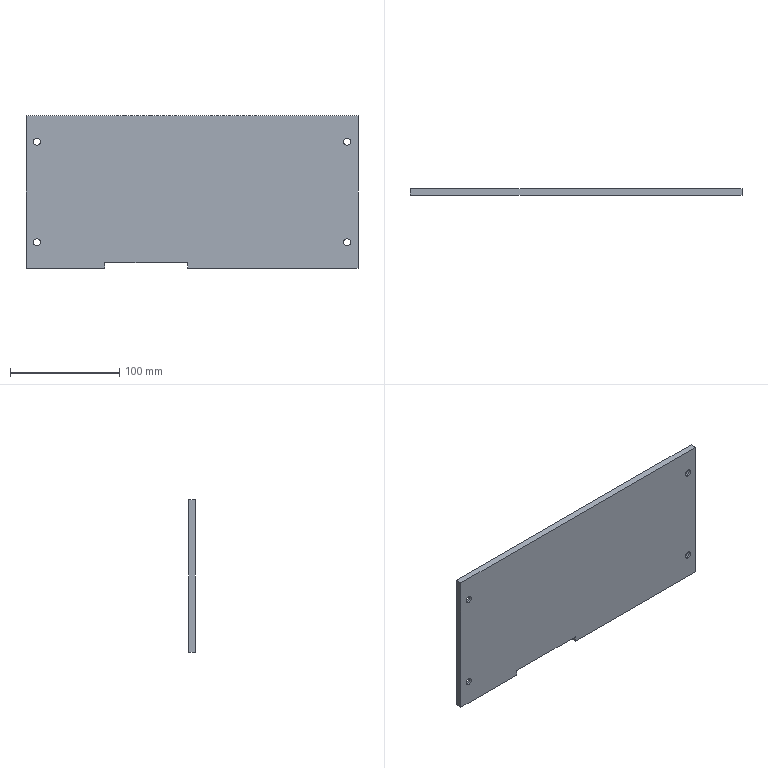Part | Creo | 1 solid | 42 faces | box 304 x 6 x 139.5 mm | volume 250207 mm3 | cone 16 | cylinder 16 | plane 10 | commonest cylinder face diameters 6.6 x8 13 x8
STEP:
#1=CARTESIAN_POINT('',(0.,0.,0.));
#2=DIRECTION('',(0.,0.,1.));
#3=DIRECTION('',(1.,0.,0.));
#4=AXIS2_PLACEMENT_3D('',#1,#2,#3);
#5=CARTESIAN_POINT('',(-4.,244.,-260.5));
#6=VERTEX_POINT('',#5);
#7=CARTESIAN_POINT('',(-4.,250.,-260.5));
#8=VERTEX_POINT('',#7);
#9=CARTESIAN_POINT('',(-4.,244.,-260.5));
#10=DIRECTION('',(0.,1.,0.));
#11=VECTOR('',#10,6.);
#12=LINE('',#9,#11);
#13=EDGE_CURVE('',#6,#8,#12,.T.);
#14=ORIENTED_EDGE('',*,*,#13,.F.);
#15=CARTESIAN_POINT('',(152.,244.,-260.5));
#16=VERTEX_POINT('',#15);
#17=CARTESIAN_POINT('',(-4.,244.,-260.5));
#18=DIRECTION('',(1.,0.,0.));
#19=VECTOR('',#18,156.);
#20=LINE('',#17,#19);
#21=EDGE_CURVE('',#6,#16,#20,.T.);
#22=ORIENTED_EDGE('',*,*,#21,.T.);
#23=CARTESIAN_POINT('',(152.,250.,-260.5));
#24=VERTEX_POINT('',#23);
#25=CARTESIAN_POINT('',(152.,244.,-260.5));
#26=DIRECTION('',(0.,1.,0.));
#27=VECTOR('',#26,6.);
#28=LINE('',#25,#27);
#29=EDGE_CURVE('',#16,#24,#28,.T.);
#30=ORIENTED_EDGE('',*,*,#29,.T.);
#31=CARTESIAN_POINT('',(152.,250.,-260.5));
#32=DIRECTION('',(-1.,0.,0.));
#33=VECTOR('',#32,156.);
#34=LINE('',#31,#33);
#35=EDGE_CURVE('',#24,#8,#34,.T.);
#36=ORIENTED_EDGE('',*,*,#35,.T.);
#37=EDGE_LOOP('',(#14,#22,#30,#36));
#38=FACE_OUTER_BOUND('',#37,.F.);
#39=CARTESIAN_POINT('',(-200.,250.,-260.5));
#40=DIRECTION('',(0.,0.,-1.));
#41=DIRECTION('',(1.,0.,0.));
#42=AXIS2_PLACEMENT_3D('',#39,#40,#41);
#43=PLANE('',#42);
#44=ADVANCED_FACE('',(#38),#43,.T.);
#45=CARTESIAN_POINT('',(-4.,244.,-255.5));
#46=VERTEX_POINT('',#45);
#47=CARTESIAN_POINT('',(-4.,244.,-255.5));
#48=DIRECTION('',(0.,0.,-1.));
#49=VECTOR('',#48,5.);
#50=LINE('',#47,#49);
#51=EDGE_CURVE('',#46,#6,#50,.T.);
#52=ORIENTED_EDGE('',*,*,#51,.T.);
#53=ORIENTED_EDGE('',*,*,#13,.T.);
#54=CARTESIAN_POINT('',(-4.,250.,-255.5));
#55=VERTEX_POINT('',#54);
#56=CARTESIAN_POINT('',(-4.,250.,-260.5));
#57=DIRECTION('',(0.,0.,1.));
#58=VECTOR('',#57,5.);
#59=LINE('',#56,#58);
#60=EDGE_CURVE('',#8,#55,#59,.T.);
#61=ORIENTED_EDGE('',*,*,#60,.T.);
#62=CARTESIAN_POINT('',(-4.,244.,-255.5));
#63=DIRECTION('',(0.,1.,0.));
#64=VECTOR('',#63,6.);
#65=LINE('',#62,#64);
#66=EDGE_CURVE('',#46,#55,#65,.T.);
#67=ORIENTED_EDGE('',*,*,#66,.F.);
#68=EDGE_LOOP('',(#52,#53,#61,#67));
#69=FACE_OUTER_BOUND('',#68,.F.);
#70=CARTESIAN_POINT('',(-4.,229.,-276.75));
#71=DIRECTION('',(1.,0.,0.));
#72=DIRECTION('',(0.,0.,-1.));
#73=AXIS2_PLACEMENT_3D('',#70,#71,#72);
#74=PLANE('',#73);
#75=ADVANCED_FACE('',(#69),#74,.F.);
#76=ORIENTED_EDGE('',*,*,#51,.F.);
#77=CARTESIAN_POINT('',(-80.,244.,-255.5));
#78=VERTEX_POINT('',#77);
#79=CARTESIAN_POINT('',(-80.,244.,-255.5));
#80=DIRECTION('',(1.,0.,0.));
#81=VECTOR('',#80,76.);
#82=LINE('',#79,#81);
#83=EDGE_CURVE('',#78,#46,#82,.T.);
#84=ORIENTED_EDGE('',*,*,#83,.F.);
#85=CARTESIAN_POINT('',(-80.,244.,-260.5));
#86=VERTEX_POINT('',#85);
#87=CARTESIAN_POINT('',(-80.,244.,-260.5));
#88=DIRECTION('',(0.,0.,1.));
#89=VECTOR('',#88,5.);
#90=LINE('',#87,#89);
#91=EDGE_CURVE('',#86,#78,#90,.T.);
#92=ORIENTED_EDGE('',*,*,#91,.F.);
#93=CARTESIAN_POINT('',(-152.,244.,-260.5));
#94=VERTEX_POINT('',#93);
#95=CARTESIAN_POINT('',(-152.,244.,-260.5));
#96=DIRECTION('',(1.,0.,0.));
#97=VECTOR('',#96,72.);
#98=LINE('',#95,#97);
#99=EDGE_CURVE('',#94,#86,#98,.T.);
#100=ORIENTED_EDGE('',*,*,#99,.F.);
#101=CARTESIAN_POINT('',(-152.,244.,-121.));
#102=VERTEX_POINT('',#101);
#103=CARTESIAN_POINT('',(-152.,244.,-121.));
#104=DIRECTION('',(0.,0.,-1.));
#105=VECTOR('',#104,139.5);
#106=LINE('',#103,#105);
#107=EDGE_CURVE('',#102,#94,#106,.T.);
#108=ORIENTED_EDGE('',*,*,#107,.F.);
#109=CARTESIAN_POINT('',(152.,244.,-121.));
#110=VERTEX_POINT('',#109);
#111=CARTESIAN_POINT('',(152.,244.,-121.));
#112=DIRECTION('',(-1.,0.,0.));
#113=VECTOR('',#112,304.);
#114=LINE('',#111,#113);
#115=EDGE_CURVE('',#110,#102,#114,.T.);
#116=ORIENTED_EDGE('',*,*,#115,.F.);
#117=CARTESIAN_POINT('',(152.,244.,-260.5));
#118=DIRECTION('',(0.,0.,1.));
#119=VECTOR('',#118,139.5);
#120=LINE('',#117,#119);
#121=EDGE_CURVE('',#16,#110,#120,.T.);
#122=ORIENTED_EDGE('',*,*,#121,.F.);
#123=ORIENTED_EDGE('',*,*,#21,.F.);
#124=EDGE_LOOP('',(#76,#84,#92,#100,#108,#116,#122,#123));
#125=FACE_OUTER_BOUND('',#124,.F.);
#126=CARTESIAN_POINT('',(-142.,244.,-240.05));
#127=VERTEX_POINT('',#126);
#128=CARTESIAN_POINT('',(-142.,244.,-233.45));
#129=VERTEX_POINT('',#128);
#130=CARTESIAN_POINT('',(-142.,244.,-236.75));
#131=DIRECTION('',(0.,1.,0.));
#132=DIRECTION('',(0.,0.,-1.));
#133=AXIS2_PLACEMENT_3D('',#130,#131,#132);
#134=CIRCLE('',#133,3.3);
#135=EDGE_CURVE('',#127,#129,#134,.T.);
#136=ORIENTED_EDGE('',*,*,#135,.F.);
#137=CARTESIAN_POINT('',(-142.,244.,-236.75));
#138=DIRECTION('',(0.,1.,0.));
#139=DIRECTION('',(0.,0.,1.));
#140=AXIS2_PLACEMENT_3D('',#137,#138,#139);
#141=CIRCLE('',#140,3.3);
#142=EDGE_CURVE('',#129,#127,#141,.T.);
#143=ORIENTED_EDGE('',*,*,#142,.F.);
#144=EDGE_LOOP('',(#136,#143));
#145=FACE_BOUND('',#144,.F.);
#146=CARTESIAN_POINT('',(-142.,244.,-148.05));
#147=VERTEX_POINT('',#146);
#148=CARTESIAN_POINT('',(-142.,244.,-141.45));
#149=VERTEX_POINT('',#148);
#150=CARTESIAN_POINT('',(-142.,244.,-144.75));
#151=DIRECTION('',(0.,1.,0.));
#152=DIRECTION('',(0.,0.,-1.));
#153=AXIS2_PLACEMENT_3D('',#150,#151,#152);
#154=CIRCLE('',#153,3.3);
#155=EDGE_CURVE('',#147,#149,#154,.T.);
#156=ORIENTED_EDGE('',*,*,#155,.F.);
#157=CARTESIAN_POINT('',(-142.,244.,-144.75));
#158=DIRECTION('',(0.,1.,0.));
#159=DIRECTION('',(0.,0.,1.));
#160=AXIS2_PLACEMENT_3D('',#157,#158,#159);
#161=CIRCLE('',#160,3.3);
#162=EDGE_CURVE('',#149,#147,#161,.T.);
#163=ORIENTED_EDGE('',*,*,#162,.F.);
#164=EDGE_LOOP('',(#156,#163));
#165=FACE_BOUND('',#164,.F.);
#166=CARTESIAN_POINT('',(142.,244.,-240.05));
#167=VERTEX_POINT('',#166);
#168=CARTESIAN_POINT('',(142.,244.,-233.45));
#169=VERTEX_POINT('',#168);
#170=CARTESIAN_POINT('',(142.,244.,-236.75));
#171=DIRECTION('',(0.,1.,0.));
#172=DIRECTION('',(0.,0.,-1.));
#173=AXIS2_PLACEMENT_3D('',#170,#171,#172);
#174=CIRCLE('',#173,3.3);
#175=EDGE_CURVE('',#167,#169,#174,.T.);
#176=ORIENTED_EDGE('',*,*,#175,.F.);
#177=CARTESIAN_POINT('',(142.,244.,-236.75));
#178=DIRECTION('',(0.,1.,0.));
#179=DIRECTION('',(0.,0.,1.));
#180=AXIS2_PLACEMENT_3D('',#177,#178,#179);
#181=CIRCLE('',#180,3.3);
#182=EDGE_CURVE('',#169,#167,#181,.T.);
#183=ORIENTED_EDGE('',*,*,#182,.F.);
#184=EDGE_LOOP('',(#176,#183));
#185=FACE_BOUND('',#184,.F.);
#186=CARTESIAN_POINT('',(142.,244.,-148.05));
#187=VERTEX_POINT('',#186);
#188=CARTESIAN_POINT('',(142.,244.,-141.45));
#189=VERTEX_POINT('',#188);
#190=CARTESIAN_POINT('',(142.,244.,-144.75));
#191=DIRECTION('',(0.,1.,0.));
#192=DIRECTION('',(0.,0.,-1.));
#193=AXIS2_PLACEMENT_3D('',#190,#191,#192);
#194=CIRCLE('',#193,3.3);
#195=EDGE_CURVE('',#187,#189,#194,.T.);
#196=ORIENTED_EDGE('',*,*,#195,.F.);
#197=CARTESIAN_POINT('',(142.,244.,-144.75));
#198=DIRECTION('',(0.,1.,0.));
#199=DIRECTION('',(0.,0.,1.));
#200=AXIS2_PLACEMENT_3D('',#197,#198,#199);
#201=CIRCLE('',#200,3.3);
#202=EDGE_CURVE('',#189,#187,#201,.T.);
#203=ORIENTED_EDGE('',*,*,#202,.F.);
#204=EDGE_LOOP('',(#196,#203));
#205=FACE_BOUND('',#204,.F.);
#206=CARTESIAN_POINT('',(0.,244.,-193.5));
#207=DIRECTION('',(0.,-1.,0.));
#208=DIRECTION('',(0.,0.,-1.));
#209=AXIS2_PLACEMENT_3D('',#206,#207,#208);
#210=PLANE('',#209);
#211=ADVANCED_FACE('',(#125,#145,#165,#185,#205),#210,.T.);
#212=ORIENTED_EDGE('',*,*,#83,.T.);
#213=ORIENTED_EDGE('',*,*,#66,.T.);
#214=CARTESIAN_POINT('',(-80.,250.,-255.5));
#215=VERTEX_POINT('',#214);
#216=CARTESIAN_POINT('',(-4.,250.,-255.5));
#217=DIRECTION('',(-1.,0.,0.));
#218=VECTOR('',#217,76.);
#219=LINE('',#216,#218);
#220=EDGE_CURVE('',#55,#215,#219,.T.);
#221=ORIENTED_EDGE('',*,*,#220,.T.);
#222=CARTESIAN_POINT('',(-80.,244.,-255.5));
#223=DIRECTION('',(0.,1.,0.));
#224=VECTOR('',#223,6.);
#225=LINE('',#222,#224);
#226=EDGE_CURVE('',#78,#215,#225,.T.);
#227=ORIENTED_EDGE('',*,*,#226,.F.);
#228=EDGE_LOOP('',(#212,#213,#221,#227));
#229=FACE_OUTER_BOUND('',#228,.F.);
#230=CARTESIAN_POINT('',(-40.75,236.,-255.5));
#231=DIRECTION('',(0.,0.,1.));
#232=DIRECTION('',(1.,0.,0.));
#233=AXIS2_PLACEMENT_3D('',#230,#231,#232);
#234=PLANE('',#233);
#235=ADVANCED_FACE('',(#229),#234,.F.);
#236=ORIENTED_EDGE('',*,*,#60,.F.);
#237=ORIENTED_EDGE('',*,*,#35,.F.);
#238=CARTESIAN_POINT('',(152.,250.,-121.));
#239=VERTEX_POINT('',#238);
#240=CARTESIAN_POINT('',(152.,250.,-121.));
#241=DIRECTION('',(0.,0.,-1.));
#242=VECTOR('',#241,139.5);
#243=LINE('',#240,#242);
#244=EDGE_CURVE('',#239,#24,#243,.T.);
#245=ORIENTED_EDGE('',*,*,#244,.F.);
#246=CARTESIAN_POINT('',(-152.,250.,-121.));
#247=VERTEX_POINT('',#246);
#248=CARTESIAN_POINT('',(-152.,250.,-121.));
#249=DIRECTION('',(1.,0.,0.));
#250=VECTOR('',#249,304.);
#251=LINE('',#248,#250);
#252=EDGE_CURVE('',#247,#239,#251,.T.);
#253=ORIENTED_EDGE('',*,*,#252,.F.);
#254=CARTESIAN_POINT('',(-152.,250.,-260.5));
#255=VERTEX_POINT('',#254);
#256=CARTESIAN_POINT('',(-152.,250.,-260.5));
#257=DIRECTION('',(0.,0.,1.));
#258=VECTOR('',#257,139.5);
#259=LINE('',#256,#258);
#260=EDGE_CURVE('',#255,#247,#259,.T.);
#261=ORIENTED_EDGE('',*,*,#260,.F.);
#262=CARTESIAN_POINT('',(-80.,250.,-260.5));
#263=VERTEX_POINT('',#262);
#264=CARTESIAN_POINT('',(-80.,250.,-260.5));
#265=DIRECTION('',(-1.,0.,0.));
#266=VECTOR('',#265,72.);
#267=LINE('',#264,#266);
#268=EDGE_CURVE('',#263,#255,#267,.T.);
#269=ORIENTED_EDGE('',*,*,#268,.F.);
#270=CARTESIAN_POINT('',(-80.,250.,-255.5));
#271=DIRECTION('',(0.,0.,-1.));
#272=VECTOR('',#271,5.);
#273=LINE('',#270,#272);
#274=EDGE_CURVE('',#215,#263,#273,.T.);
#275=ORIENTED_EDGE('',*,*,#274,.F.);
#276=ORIENTED_EDGE('',*,*,#220,.F.);
#277=EDGE_LOOP('',(#236,#237,#245,#253,#261,#269,#275,#276));
#278=FACE_OUTER_BOUND('',#277,.F.);
#279=CARTESIAN_POINT('',(-142.,250.,-243.5));
#280=VERTEX_POINT('',#279);
#281=CARTESIAN_POINT('',(-142.,250.,-230.));
#282=VERTEX_POINT('',#281);
#283=CARTESIAN_POINT('',(-142.,250.,-236.75));
#284=DIRECTION('',(0.,-1.,0.));
#285=DIRECTION('',(0.,0.,-1.));
#286=AXIS2_PLACEMENT_3D('',#283,#284,#285);
#287=CIRCLE('',#286,6.75);
#288=EDGE_CURVE('',#280,#282,#287,.T.);
#289=ORIENTED_EDGE('',*,*,#288,.F.);
#290=CARTESIAN_POINT('',(-142.,250.,-236.75));
#291=DIRECTION('',(0.,-1.,0.));
#292=DIRECTION('',(0.,0.,1.));
#293=AXIS2_PLACEMENT_3D('',#290,#291,#292);
#294=CIRCLE('',#293,6.75);
#295=EDGE_CURVE('',#282,#280,#294,.T.);
#296=ORIENTED_EDGE('',*,*,#295,.F.);
#297=EDGE_LOOP('',(#289,#296));
#298=FACE_BOUND('',#297,.F.);
#299=CARTESIAN_POINT('',(-142.,250.,-151.5));
#300=VERTEX_POINT('',#299);
#301=CARTESIAN_POINT('',(-142.,250.,-138.));
#302=VERTEX_POINT('',#301);
#303=CARTESIAN_POINT('',(-142.,250.,-144.75));
#304=DIRECTION('',(0.,-1.,0.));
#305=DIRECTION('',(0.,0.,-1.));
#306=AXIS2_PLACEMENT_3D('',#303,#304,#305);
#307=CIRCLE('',#306,6.75);
#308=EDGE_CURVE('',#300,#302,#307,.T.);
#309=ORIENTED_EDGE('',*,*,#308,.F.);
#310=CARTESIAN_POINT('',(-142.,250.,-144.75));
#311=DIRECTION('',(0.,-1.,0.));
#312=DIRECTION('',(0.,0.,1.));
#313=AXIS2_PLACEMENT_3D('',#310,#311,#312);
#314=CIRCLE('',#313,6.75);
#315=EDGE_CURVE('',#302,#300,#314,.T.);
#316=ORIENTED_EDGE('',*,*,#315,.F.);
#317=EDGE_LOOP('',(#309,#316));
#318=FACE_BOUND('',#317,.F.);
#319=CARTESIAN_POINT('',(142.,250.,-243.5));
#320=VERTEX_POINT('',#319);
#321=CARTESIAN_POINT('',(142.,250.,-230.));
#322=VERTEX_POINT('',#321);
#323=CARTESIAN_POINT('',(142.,250.,-236.75));
#324=DIRECTION('',(0.,-1.,0.));
#325=DIRECTION('',(0.,0.,-1.));
#326=AXIS2_PLACEMENT_3D('',#323,#324,#325);
#327=CIRCLE('',#326,6.75);
#328=EDGE_CURVE('',#320,#322,#327,.T.);
#329=ORIENTED_EDGE('',*,*,#328,.F.);
#330=CARTESIAN_POINT('',(142.,250.,-236.75));
#331=DIRECTION('',(0.,-1.,0.));
#332=DIRECTION('',(0.,0.,1.));
#333=AXIS2_PLACEMENT_3D('',#330,#331,#332);
#334=CIRCLE('',#333,6.75);
#335=EDGE_CURVE('',#322,#320,#334,.T.);
#336=ORIENTED_EDGE('',*,*,#335,.F.);
#337=EDGE_LOOP('',(#329,#336));
#338=FACE_BOUND('',#337,.F.);
#339=CARTESIAN_POINT('',(142.,250.,-151.5));
#340=VERTEX_POINT('',#339);
#341=CARTESIAN_POINT('',(142.,250.,-138.));
#342=VERTEX_POINT('',#341);
#343=CARTESIAN_POINT('',(142.,250.,-144.75));
#344=DIRECTION('',(0.,-1.,0.));
#345=DIRECTION('',(0.,0.,-1.));
#346=AXIS2_PLACEMENT_3D('',#343,#344,#345);
#347=CIRCLE('',#346,6.75);
#348=EDGE_CURVE('',#340,#342,#347,.T.);
#349=ORIENTED_EDGE('',*,*,#348,.F.);
#350=CARTESIAN_POINT('',(142.,250.,-144.75));
#351=DIRECTION('',(0.,-1.,0.));
#352=DIRECTION('',(0.,0.,1.));
#353=AXIS2_PLACEMENT_3D('',#350,#351,#352);
#354=CIRCLE('',#353,6.75);
#355=EDGE_CURVE('',#342,#340,#354,.T.);
#356=ORIENTED_EDGE('',*,*,#355,.F.);
#357=EDGE_LOOP('',(#349,#356));
#358=FACE_BOUND('',#357,.F.);
#359=CARTESIAN_POINT('',(-200.,250.,-260.5));
#360=DIRECTION('',(0.,-1.,0.));
#361=DIRECTION('',(0.,0.,1.));
#362=AXIS2_PLACEMENT_3D('',#359,#360,#361);
#363=PLANE('',#362);
#364=ADVANCED_FACE('',(#278,#298,#318,#338,#358),#363,.F.);
#365=ORIENTED_EDGE('',*,*,#244,.T.);
#366=ORIENTED_EDGE('',*,*,#29,.F.);
#367=ORIENTED_EDGE('',*,*,#121,.T.);
#368=CARTESIAN_POINT('',(152.,244.,-121.));
#369=DIRECTION('',(0.,1.,0.));
#370=VECTOR('',#369,6.);
#371=LINE('',#368,#370);
#372=EDGE_CURVE('',#110,#239,#371,.T.);
#373=ORIENTED_EDGE('',*,*,#372,.T.);
#374=EDGE_LOOP('',(#365,#366,#367,#373));
#375=FACE_OUTER_BOUND('',#374,.F.);
#376=CARTESIAN_POINT('',(152.,-250.,-260.5));
#377=DIRECTION('',(1.,0.,0.));
#378=DIRECTION('',(0.,0.,1.));
#379=AXIS2_PLACEMENT_3D('',#376,#377,#378);
#380=PLANE('',#379);
#381=ADVANCED_FACE('',(#375),#380,.T.);
#382=CARTESIAN_POINT('',(-152.,244.,-121.));
#383=DIRECTION('',(0.,1.,0.));
#384=VECTOR('',#383,6.);
#385=LINE('',#382,#384);
#386=EDGE_CURVE('',#102,#247,#385,.T.);
#387=ORIENTED_EDGE('',*,*,#386,.T.);
#388=ORIENTED_EDGE('',*,*,#252,.T.);
#389=ORIENTED_EDGE('',*,*,#372,.F.);
#390=ORIENTED_EDGE('',*,*,#115,.T.);
#391=EDGE_LOOP('',(#387,#388,#389,#390));
#392=FACE_OUTER_BOUND('',#391,.F.);
#393=CARTESIAN_POINT('',(-200.,250.,-121.));
#394=DIRECTION('',(0.,0.,-1.));
#395=DIRECTION('',(1.,0.,0.));
#396=AXIS2_PLACEMENT_3D('',#393,#394,#395);
#397=PLANE('',#396);
#398=ADVANCED_FACE('',(#392),#397,.F.);
#399=CARTESIAN_POINT('',(-152.,244.,-260.5));
#400=DIRECTION('',(0.,1.,0.));
#401=VECTOR('',#400,6.);
#402=LINE('',#399,#401);
#403=EDGE_CURVE('',#94,#255,#402,.T.);
#404=ORIENTED_EDGE('',*,*,#403,.T.);
#405=ORIENTED_EDGE('',*,*,#260,.T.);
#406=ORIENTED_EDGE('',*,*,#386,.F.);
#407=ORIENTED_EDGE('',*,*,#107,.T.);
#408=EDGE_LOOP('',(#404,#405,#406,#407));
#409=FACE_OUTER_BOUND('',#408,.F.);
#410=CARTESIAN_POINT('',(-152.,250.,-260.5));
#411=DIRECTION('',(-1.,0.,0.));
#412=DIRECTION('',(0.,1.,0.));
#413=AXIS2_PLACEMENT_3D('',#410,#411,#412);
#414=PLANE('',#413);
#415=ADVANCED_FACE('',(#409),#414,.T.);
#416=CARTESIAN_POINT('',(-80.,250.,-260.5));
#417=DIRECTION('',(0.,-1.,0.));
#418=VECTOR('',#417,6.);
#419=LINE('',#416,#418);
#420=EDGE_CURVE('',#263,#86,#419,.T.);
#421=ORIENTED_EDGE('',*,*,#420,.F.);
#422=ORIENTED_EDGE('',*,*,#268,.T.);
#423=ORIENTED_EDGE('',*,*,#403,.F.);
#424=ORIENTED_EDGE('',*,*,#99,.T.);
#425=EDGE_LOOP('',(#421,#422,#423,#424));
#426=FACE_OUTER_BOUND('',#425,.F.);
#427=CARTESIAN_POINT('',(-200.,250.,-260.5));
#428=DIRECTION('',(0.,0.,-1.));
#429=DIRECTION('',(1.,0.,0.));
#430=AXIS2_PLACEMENT_3D('',#427,#428,#429);
#431=PLANE('',#430);
#432=ADVANCED_FACE('',(#426),#431,.T.);
#433=ORIENTED_EDGE('',*,*,#91,.T.);
#434=ORIENTED_EDGE('',*,*,#226,.T.);
#435=ORIENTED_EDGE('',*,*,#274,.T.);
#436=ORIENTED_EDGE('',*,*,#420,.T.);
#437=EDGE_LOOP('',(#433,#434,#435,#436));
#438=FACE_OUTER_BOUND('',#437,.F.);
#439=CARTESIAN_POINT('',(-80.,229.,-276.75));
#440=DIRECTION('',(-1.,0.,0.));
#441=DIRECTION('',(0.,0.,1.));
#442=AXIS2_PLACEMENT_3D('',#439,#440,#441);
#443=PLANE('',#442);
#444=ADVANCED_FACE('',(#438),#443,.F.);
#445=ORIENTED_EDGE('',*,*,#288,.T.);
#446=CARTESIAN_POINT('',(-142.,249.75,-230.25));
#447=VERTEX_POINT('',#446);
#448=CARTESIAN_POINT('',(-142.,249.75,-230.25));
#449=DIRECTION('',(0.,0.7071,0.7071));
#450=VECTOR('',#449,0.3536);
#451=LINE('',#448,#450);
#452=EDGE_CURVE('',#447,#282,#451,.T.);
#453=ORIENTED_EDGE('',*,*,#452,.F.);
#454=CARTESIAN_POINT('',(-135.5,249.75,-236.75));
#455=VERTEX_POINT('',#454);
#456=CARTESIAN_POINT('',(-142.,249.75,-236.75));
#457=DIRECTION('',(0.,-1.,0.));
#458=DIRECTION('',(1.,0.,0.));
#459=AXIS2_PLACEMENT_3D('',#456,#457,#458);
#460=CIRCLE('',#459,6.5);
#461=EDGE_CURVE('',#455,#447,#460,.T.);
#462=ORIENTED_EDGE('',*,*,#461,.F.);
#463=CARTESIAN_POINT('',(-142.,249.75,-243.25));
#464=VERTEX_POINT('',#463);
#465=CARTESIAN_POINT('',(-142.,249.75,-236.75));
#466=DIRECTION('',(0.,-1.,0.));
#467=DIRECTION('',(0.,0.,-1.));
#468=AXIS2_PLACEMENT_3D('',#465,#466,#467);
#469=CIRCLE('',#468,6.5);
#470=EDGE_CURVE('',#464,#455,#469,.T.);
#471=ORIENTED_EDGE('',*,*,#470,.F.);
#472=CARTESIAN_POINT('',(-142.,249.75,-243.25));
#473=DIRECTION('',(0.,0.7071,-0.7071));
#474=VECTOR('',#473,0.3536);
#475=LINE('',#472,#474);
#476=EDGE_CURVE('',#464,#280,#475,.T.);
#477=ORIENTED_EDGE('',*,*,#476,.T.);
#478=EDGE_LOOP('',(#445,#453,#462,#471,#477));
#479=FACE_OUTER_BOUND('',#478,.F.);
#480=CARTESIAN_POINT('',(-142.,249.875,-236.75));
#481=DIRECTION('',(0.,1.,0.));
#482=DIRECTION('',(0.,0.,1.));
#483=AXIS2_PLACEMENT_3D('',#480,#481,#482);
#484=CONICAL_SURFACE('',#483,6.625,45.);
#485=ADVANCED_FACE('',(#479),#484,.F.);
#486=ORIENTED_EDGE('',*,*,#295,.T.);
#487=ORIENTED_EDGE('',*,*,#476,.F.);
#488=CARTESIAN_POINT('',(-148.5,249.75,-236.75));
#489=VERTEX_POINT('',#488);
#490=CARTESIAN_POINT('',(-142.,249.75,-236.75));
#491=DIRECTION('',(0.,-1.,0.));
#492=DIRECTION('',(-1.,0.,0.));
#493=AXIS2_PLACEMENT_3D('',#490,#491,#492);
#494=CIRCLE('',#493,6.5);
#495=EDGE_CURVE('',#489,#464,#494,.T.);
#496=ORIENTED_EDGE('',*,*,#495,.F.);
#497=CARTESIAN_POINT('',(-142.,249.75,-236.75));
#498=DIRECTION('',(0.,-1.,0.));
#499=DIRECTION('',(0.,0.,1.));
#500=AXIS2_PLACEMENT_3D('',#497,#498,#499);
#501=CIRCLE('',#500,6.5);
#502=EDGE_CURVE('',#447,#489,#501,.T.);
#503=ORIENTED_EDGE('',*,*,#502,.F.);
#504=ORIENTED_EDGE('',*,*,#452,.T.);
#505=EDGE_LOOP('',(#486,#487,#496,#503,#504));
#506=FACE_OUTER_BOUND('',#505,.F.);
#507=CARTESIAN_POINT('',(-142.,249.875,-236.75));
#508=DIRECTION('',(0.,1.,0.));
#509=DIRECTION('',(0.,0.,1.));
#510=AXIS2_PLACEMENT_3D('',#507,#508,#509);
#511=CONICAL_SURFACE('',#510,6.625,45.);
#512=ADVANCED_FACE('',(#506),#511,.F.);
#513=CARTESIAN_POINT('',(-135.5,248.26,-236.75));
#514=VERTEX_POINT('',#513);
#515=CARTESIAN_POINT('',(-148.5,248.26,-236.75));
#516=VERTEX_POINT('',#515);
#517=CARTESIAN_POINT('',(-142.,248.26,-236.75));
#518=DIRECTION('',(0.,1.,0.));
#519=DIRECTION('',(1.,0.,0.));
#520=AXIS2_PLACEMENT_3D('',#517,#518,#519);
#521=CIRCLE('',#520,6.5);
#522=EDGE_CURVE('',#514,#516,#521,.T.);
#523=ORIENTED_EDGE('',*,*,#522,.T.);
#524=CARTESIAN_POINT('',(-148.5,248.26,-236.75));
#525=DIRECTION('',(0.,1.,0.));
#526=VECTOR('',#525,1.49);
#527=LINE('',#524,#526);
#528=EDGE_CURVE('',#516,#489,#527,.T.);
#529=ORIENTED_EDGE('',*,*,#528,.T.);
#530=ORIENTED_EDGE('',*,*,#495,.T.);
#531=ORIENTED_EDGE('',*,*,#470,.T.);
#532=CARTESIAN_POINT('',(-135.5,248.26,-236.75));
#533=DIRECTION('',(0.,1.,0.));
#534=VECTOR('',#533,1.49);
#535=LINE('',#532,#534);
#536=EDGE_CURVE('',#514,#455,#535,.T.);
#537=ORIENTED_EDGE('',*,*,#536,.F.);
#538=EDGE_LOOP('',(#523,#529,#530,#531,#537));
#539=FACE_OUTER_BOUND('',#538,.F.);
#540=CARTESIAN_POINT('',(-142.,250.,-236.75));
#541=DIRECTION('',(0.,1.,0.));
#542=DIRECTION('',(1.,0.,0.));
#543=AXIS2_PLACEMENT_3D('',#540,#541,#542);
#544=CYLINDRICAL_SURFACE('',#543,6.5);
#545=ADVANCED_FACE('',(#539),#544,.F.);
#546=ORIENTED_EDGE('',*,*,#522,.F.);
#547=CARTESIAN_POINT('',(-138.7,245.7,-236.75));
#548=VERTEX_POINT('',#547);
#549=CARTESIAN_POINT('',(-138.7,245.7,-236.75));
#550=DIRECTION('',(0.7809,0.6247,0.));
#551=VECTOR('',#550,4.098);
#552=LINE('',#549,#551);
#553=EDGE_CURVE('',#548,#514,#552,.T.);
#554=ORIENTED_EDGE('',*,*,#553,.F.);
#555=CARTESIAN_POINT('',(-142.,245.7,-240.05));
#556=VERTEX_POINT('',#555);
#557=CARTESIAN_POINT('',(-142.,245.7,-236.75));
#558=DIRECTION('',(0.,-1.,0.));
#559=DIRECTION('',(0.,0.,-1.));
#560=AXIS2_PLACEMENT_3D('',#557,#558,#559);
#561=CIRCLE('',#560,3.3);
#562=EDGE_CURVE('',#556,#548,#561,.T.);
#563=ORIENTED_EDGE('',*,*,#562,.F.);
#564=CARTESIAN_POINT('',(-145.3,245.7,-236.75));
#565=VERTEX_POINT('',#564);
#566=CARTESIAN_POINT('',(-142.,245.7,-236.75));
#567=DIRECTION('',(0.,-1.,0.));
#568=DIRECTION('',(-1.,0.,0.));
#569=AXIS2_PLACEMENT_3D('',#566,#567,#568);
#570=CIRCLE('',#569,3.3);
#571=EDGE_CURVE('',#565,#556,#570,.T.);
#572=ORIENTED_EDGE('',*,*,#571,.F.);
#573=CARTESIAN_POINT('',(-145.3,245.7,-236.75));
#574=DIRECTION('',(-0.7809,0.6247,0.));
#575=VECTOR('',#574,4.098);
#576=LINE('',#573,#575);
#577=EDGE_CURVE('',#565,#516,#576,.T.);
#578=ORIENTED_EDGE('',*,*,#577,.T.);
#579=EDGE_LOOP('',(#546,#554,#563,#572,#578));
#580=FACE_OUTER_BOUND('',#579,.F.);
#581=CARTESIAN_POINT('',(-142.,246.98,-236.75));
#582=DIRECTION('',(0.,1.,0.));
#583=DIRECTION('',(1.,0.,0.));
#584=AXIS2_PLACEMENT_3D('',#581,#582,#583);
#585=CONICAL_SURFACE('',#584,4.9,51.34);
#586=ADVANCED_FACE('',(#580),#585,.F.);
#587=CARTESIAN_POINT('',(-142.,248.26,-236.75));
#588=DIRECTION('',(0.,1.,0.));
#589=DIRECTION('',(-1.,0.,0.));
#590=AXIS2_PLACEMENT_3D('',#587,#588,#589);
#591=CIRCLE('',#590,6.5);
#592=EDGE_CURVE('',#516,#514,#591,.T.);
#593=ORIENTED_EDGE('',*,*,#592,.F.);
#594=ORIENTED_EDGE('',*,*,#577,.F.);
#595=CARTESIAN_POINT('',(-142.,245.7,-233.45));
#596=VERTEX_POINT('',#595);
#597=CARTESIAN_POINT('',(-142.,245.7,-236.75));
#598=DIRECTION('',(0.,-1.,0.));
#599=DIRECTION('',(0.,0.,1.));
#600=AXIS2_PLACEMENT_3D('',#597,#598,#599);
#601=CIRCLE('',#600,3.3);
#602=EDGE_CURVE('',#596,#565,#601,.T.);
#603=ORIENTED_EDGE('',*,*,#602,.F.);
#604=CARTESIAN_POINT('',(-142.,245.7,-236.75));
#605=DIRECTION('',(0.,-1.,0.));
#606=DIRECTION('',(1.,0.,0.));
#607=AXIS2_PLACEMENT_3D('',#604,#605,#606);
#608=CIRCLE('',#607,3.3);
#609=EDGE_CURVE('',#548,#596,#608,.T.);
#610=ORIENTED_EDGE('',*,*,#609,.F.);
#611=ORIENTED_EDGE('',*,*,#553,.T.);
#612=EDGE_LOOP('',(#593,#594,#603,#610,#611));
#613=FACE_OUTER_BOUND('',#612,.F.);
#614=CARTESIAN_POINT('',(-142.,246.98,-236.75));
#615=DIRECTION('',(0.,1.,0.));
#616=DIRECTION('',(1.,0.,0.));
#617=AXIS2_PLACEMENT_3D('',#614,#615,#616);
#618=CONICAL_SURFACE('',#617,4.9,51.34);
#619=ADVANCED_FACE('',(#613),#618,.F.);
#620=ORIENTED_EDGE('',*,*,#592,.T.);
#621=ORIENTED_EDGE('',*,*,#536,.T.);
#622=ORIENTED_EDGE('',*,*,#461,.T.);
#623=ORIENTED_EDGE('',*,*,#502,.T.);
#624=ORIENTED_EDGE('',*,*,#528,.F.);
#625=EDGE_LOOP('',(#620,#621,#622,#623,#624));
#626=FACE_OUTER_BOUND('',#625,.F.);
#627=CARTESIAN_POINT('',(-142.,250.,-236.75));
#628=DIRECTION('',(0.,1.,0.));
#629=DIRECTION('',(1.,0.,0.));
#630=AXIS2_PLACEMENT_3D('',#627,#628,#629);
#631=CYLINDRICAL_SURFACE('',#630,6.5);
#632=ADVANCED_FACE('',(#626),#631,.F.);
#633=ORIENTED_EDGE('',*,*,#135,.T.);
#634=CARTESIAN_POINT('',(-142.,245.7,-233.45));
#635=DIRECTION('',(0.,-1.,0.));
#636=VECTOR('',#635,1.7);
#637=LINE('',#634,#636);
#638=EDGE_CURVE('',#596,#129,#637,.T.);
#639=ORIENTED_EDGE('',*,*,#638,.F.);
#640=ORIENTED_EDGE('',*,*,#602,.T.);
#641=ORIENTED_EDGE('',*,*,#571,.T.);
#642=CARTESIAN_POINT('',(-142.,245.7,-240.05));
#643=DIRECTION('',(0.,-1.,0.));
#644=VECTOR('',#643,1.7);
#645=LINE('',#642,#644);
#646=EDGE_CURVE('',#556,#127,#645,.T.);
#647=ORIENTED_EDGE('',*,*,#646,.T.);
#648=EDGE_LOOP('',(#633,#639,#640,#641,#647));
#649=FACE_OUTER_BOUND('',#648,.F.);
#650=CARTESIAN_POINT('',(-142.,200.,-236.75));
#651=DIRECTION('',(0.,-1.,0.));
#652=DIRECTION('',(0.,0.,-1.));
#653=AXIS2_PLACEMENT_3D('',#650,#651,#652);
#654=CYLINDRICAL_SURFACE('',#653,3.3);
#655=ADVANCED_FACE('',(#649),#654,.F.);
#656=ORIENTED_EDGE('',*,*,#142,.T.);
#657=ORIENTED_EDGE('',*,*,#646,.F.);
#658=ORIENTED_EDGE('',*,*,#562,.T.);
#659=ORIENTED_EDGE('',*,*,#609,.T.);
#660=ORIENTED_EDGE('',*,*,#638,.T.);
#661=EDGE_LOOP('',(#656,#657,#658,#659,#660));
#662=FACE_OUTER_BOUND('',#661,.F.);
#663=CARTESIAN_POINT('',(-142.,200.,-236.75));
#664=DIRECTION('',(0.,-1.,0.));
#665=DIRECTION('',(0.,0.,-1.));
#666=AXIS2_PLACEMENT_3D('',#663,#664,#665);
#667=CYLINDRICAL_SURFACE('',#666,3.3);
#668=ADVANCED_FACE('',(#662),#667,.F.);
#669=ORIENTED_EDGE('',*,*,#308,.T.);
#670=CARTESIAN_POINT('',(-142.,249.75,-138.25));
#671=VERTEX_POINT('',#670);
#672=CARTESIAN_POINT('',(-142.,249.75,-138.25));
#673=DIRECTION('',(0.,0.7071,0.7071));
#674=VECTOR('',#673,0.3536);
#675=LINE('',#672,#674);
#676=EDGE_CURVE('',#671,#302,#675,.T.);
#677=ORIENTED_EDGE('',*,*,#676,.F.);
#678=CARTESIAN_POINT('',(-135.5,249.75,-144.75));
#679=VERTEX_POINT('',#678);
#680=CARTESIAN_POINT('',(-142.,249.75,-144.75));
#681=DIRECTION('',(0.,-1.,0.));
#682=DIRECTION('',(1.,0.,0.));
#683=AXIS2_PLACEMENT_3D('',#680,#681,#682);
#684=CIRCLE('',#683,6.5);
#685=EDGE_CURVE('',#679,#671,#684,.T.);
#686=ORIENTED_EDGE('',*,*,#685,.F.);
#687=CARTESIAN_POINT('',(-142.,249.75,-151.25));
#688=VERTEX_POINT('',#687);
#689=CARTESIAN_POINT('',(-142.,249.75,-144.75));
#690=DIRECTION('',(0.,-1.,0.));
#691=DIRECTION('',(0.,0.,-1.));
#692=AXIS2_PLACEMENT_3D('',#689,#690,#691);
#693=CIRCLE('',#692,6.5);
#694=EDGE_CURVE('',#688,#679,#693,.T.);
#695=ORIENTED_EDGE('',*,*,#694,.F.);
#696=CARTESIAN_POINT('',(-142.,249.75,-151.25));
#697=DIRECTION('',(0.,0.7071,-0.7071));
#698=VECTOR('',#697,0.3536);
#699=LINE('',#696,#698);
#700=EDGE_CURVE('',#688,#300,#699,.T.);
#701=ORIENTED_EDGE('',*,*,#700,.T.);
#702=EDGE_LOOP('',(#669,#677,#686,#695,#701));
#703=FACE_OUTER_BOUND('',#702,.F.);
#704=CARTESIAN_POINT('',(-142.,249.875,-144.75));
#705=DIRECTION('',(0.,1.,0.));
#706=DIRECTION('',(0.,0.,1.));
#707=AXIS2_PLACEMENT_3D('',#704,#705,#706);
#708=CONICAL_SURFACE('',#707,6.625,45.);
#709=ADVANCED_FACE('',(#703),#708,.F.);
#710=ORIENTED_EDGE('',*,*,#315,.T.);
#711=ORIENTED_EDGE('',*,*,#700,.F.);
#712=CARTESIAN_POINT('',(-148.5,249.75,-144.75));
#713=VERTEX_POINT('',#712);
#714=CARTESIAN_POINT('',(-142.,249.75,-144.75));
#715=DIRECTION('',(0.,-1.,0.));
#716=DIRECTION('',(-1.,0.,0.));
#717=AXIS2_PLACEMENT_3D('',#714,#715,#716);
#718=CIRCLE('',#717,6.5);
#719=EDGE_CURVE('',#713,#688,#718,.T.);
#720=ORIENTED_EDGE('',*,*,#719,.F.);
#721=CARTESIAN_POINT('',(-142.,249.75,-144.75));
#722=DIRECTION('',(0.,-1.,0.));
#723=DIRECTION('',(0.,0.,1.));
#724=AXIS2_PLACEMENT_3D('',#721,#722,#723);
#725=CIRCLE('',#724,6.5);
#726=EDGE_CURVE('',#671,#713,#725,.T.);
#727=ORIENTED_EDGE('',*,*,#726,.F.);
#728=ORIENTED_EDGE('',*,*,#676,.T.);
#729=EDGE_LOOP('',(#710,#711,#720,#727,#728));
#730=FACE_OUTER_BOUND('',#729,.F.);
#731=CARTESIAN_POINT('',(-142.,249.875,-144.75));
#732=DIRECTION('',(0.,1.,0.));
#733=DIRECTION('',(0.,0.,1.));
#734=AXIS2_PLACEMENT_3D('',#731,#732,#733);
#735=CONICAL_SURFACE('',#734,6.625,45.);
#736=ADVANCED_FACE('',(#730),#735,.F.);
#737=CARTESIAN_POINT('',(-135.5,248.26,-144.75));
#738=VERTEX_POINT('',#737);
#739=CARTESIAN_POINT('',(-148.5,248.26,-144.75));
#740=VERTEX_POINT('',#739);
#741=CARTESIAN_POINT('',(-142.,248.26,-144.75));
#742=DIRECTION('',(0.,1.,0.));
#743=DIRECTION('',(1.,0.,0.));
#744=AXIS2_PLACEMENT_3D('',#741,#742,#743);
#745=CIRCLE('',#744,6.5);
#746=EDGE_CURVE('',#738,#740,#745,.T.);
#747=ORIENTED_EDGE('',*,*,#746,.T.);
#748=CARTESIAN_POINT('',(-148.5,248.26,-144.75));
#749=DIRECTION('',(0.,1.,0.));
#750=VECTOR('',#749,1.49);
#751=LINE('',#748,#750);
#752=EDGE_CURVE('',#740,#713,#751,.T.);
#753=ORIENTED_EDGE('',*,*,#752,.T.);
#754=ORIENTED_EDGE('',*,*,#719,.T.);
#755=ORIENTED_EDGE('',*,*,#694,.T.);
#756=CARTESIAN_POINT('',(-135.5,248.26,-144.75));
#757=DIRECTION('',(0.,1.,0.));
#758=VECTOR('',#757,1.49);
#759=LINE('',#756,#758);
#760=EDGE_CURVE('',#738,#679,#759,.T.);
#761=ORIENTED_EDGE('',*,*,#760,.F.);
#762=EDGE_LOOP('',(#747,#753,#754,#755,#761));
#763=FACE_OUTER_BOUND('',#762,.F.);
#764=CARTESIAN_POINT('',(-142.,250.,-144.75));
#765=DIRECTION('',(0.,1.,0.));
#766=DIRECTION('',(1.,0.,0.));
#767=AXIS2_PLACEMENT_3D('',#764,#765,#766);
#768=CYLINDRICAL_SURFACE('',#767,6.5);
#769=ADVANCED_FACE('',(#763),#768,.F.);
#770=ORIENTED_EDGE('',*,*,#746,.F.);
#771=CARTESIAN_POINT('',(-138.7,245.7,-144.75));
#772=VERTEX_POINT('',#771);
#773=CARTESIAN_POINT('',(-138.7,245.7,-144.75));
#774=DIRECTION('',(0.7809,0.6247,0.));
#775=VECTOR('',#774,4.098);
#776=LINE('',#773,#775);
#777=EDGE_CURVE('',#772,#738,#776,.T.);
#778=ORIENTED_EDGE('',*,*,#777,.F.);
#779=CARTESIAN_POINT('',(-142.,245.7,-148.05));
#780=VERTEX_POINT('',#779);
#781=CARTESIAN_POINT('',(-142.,245.7,-144.75));
#782=DIRECTION('',(0.,-1.,0.));
#783=DIRECTION('',(0.,0.,-1.));
#784=AXIS2_PLACEMENT_3D('',#781,#782,#783);
#785=CIRCLE('',#784,3.3);
#786=EDGE_CURVE('',#780,#772,#785,.T.);
#787=ORIENTED_EDGE('',*,*,#786,.F.);
#788=CARTESIAN_POINT('',(-145.3,245.7,-144.75));
#789=VERTEX_POINT('',#788);
#790=CARTESIAN_POINT('',(-142.,245.7,-144.75));
#791=DIRECTION('',(0.,-1.,0.));
#792=DIRECTION('',(-1.,0.,0.));
#793=AXIS2_PLACEMENT_3D('',#790,#791,#792);
#794=CIRCLE('',#793,3.3);
#795=EDGE_CURVE('',#789,#780,#794,.T.);
#796=ORIENTED_EDGE('',*,*,#795,.F.);
#797=CARTESIAN_POINT('',(-145.3,245.7,-144.75));
#798=DIRECTION('',(-0.7809,0.6247,0.));
#799=VECTOR('',#798,4.098);
#800=LINE('',#797,#799);
#801=EDGE_CURVE('',#789,#740,#800,.T.);
#802=ORIENTED_EDGE('',*,*,#801,.T.);
#803=EDGE_LOOP('',(#770,#778,#787,#796,#802));
#804=FACE_OUTER_BOUND('',#803,.F.);
#805=CARTESIAN_POINT('',(-142.,246.98,-144.75));
#806=DIRECTION('',(0.,1.,0.));
#807=DIRECTION('',(1.,0.,0.));
#808=AXIS2_PLACEMENT_3D('',#805,#806,#807);
#809=CONICAL_SURFACE('',#808,4.9,51.34);
#810=ADVANCED_FACE('',(#804),#809,.F.);
#811=CARTESIAN_POINT('',(-142.,248.26,-144.75));
#812=DIRECTION('',(0.,1.,0.));
#813=DIRECTION('',(-1.,0.,0.));
#814=AXIS2_PLACEMENT_3D('',#811,#812,#813);
#815=CIRCLE('',#814,6.5);
#816=EDGE_CURVE('',#740,#738,#815,.T.);
#817=ORIENTED_EDGE('',*,*,#816,.F.);
#818=ORIENTED_EDGE('',*,*,#801,.F.);
#819=CARTESIAN_POINT('',(-142.,245.7,-141.45));
#820=VERTEX_POINT('',#819);
#821=CARTESIAN_POINT('',(-142.,245.7,-144.75));
#822=DIRECTION('',(0.,-1.,0.));
#823=DIRECTION('',(0.,0.,1.));
#824=AXIS2_PLACEMENT_3D('',#821,#822,#823);
#825=CIRCLE('',#824,3.3);
#826=EDGE_CURVE('',#820,#789,#825,.T.);
#827=ORIENTED_EDGE('',*,*,#826,.F.);
#828=CARTESIAN_POINT('',(-142.,245.7,-144.75));
#829=DIRECTION('',(0.,-1.,0.));
#830=DIRECTION('',(1.,0.,0.));
#831=AXIS2_PLACEMENT_3D('',#828,#829,#830);
#832=CIRCLE('',#831,3.3);
#833=EDGE_CURVE('',#772,#820,#832,.T.);
#834=ORIENTED_EDGE('',*,*,#833,.F.);
#835=ORIENTED_EDGE('',*,*,#777,.T.);
#836=EDGE_LOOP('',(#817,#818,#827,#834,#835));
#837=FACE_OUTER_BOUND('',#836,.F.);
#838=CARTESIAN_POINT('',(-142.,246.98,-144.75));
#839=DIRECTION('',(0.,1.,0.));
#840=DIRECTION('',(1.,0.,0.));
#841=AXIS2_PLACEMENT_3D('',#838,#839,#840);
#842=CONICAL_SURFACE('',#841,4.9,51.34);
#843=ADVANCED_FACE('',(#837),#842,.F.);
#844=ORIENTED_EDGE('',*,*,#816,.T.);
#845=ORIENTED_EDGE('',*,*,#760,.T.);
#846=ORIENTED_EDGE('',*,*,#685,.T.);
#847=ORIENTED_EDGE('',*,*,#726,.T.);
#848=ORIENTED_EDGE('',*,*,#752,.F.);
#849=EDGE_LOOP('',(#844,#845,#846,#847,#848));
#850=FACE_OUTER_BOUND('',#849,.F.);
#851=CARTESIAN_POINT('',(-142.,250.,-144.75));
#852=DIRECTION('',(0.,1.,0.));
#853=DIRECTION('',(1.,0.,0.));
#854=AXIS2_PLACEMENT_3D('',#851,#852,#853);
#855=CYLINDRICAL_SURFACE('',#854,6.5);
#856=ADVANCED_FACE('',(#850),#855,.F.);
#857=ORIENTED_EDGE('',*,*,#155,.T.);
#858=CARTESIAN_POINT('',(-142.,245.7,-141.45));
#859=DIRECTION('',(0.,-1.,0.));
#860=VECTOR('',#859,1.7);
#861=LINE('',#858,#860);
#862=EDGE_CURVE('',#820,#149,#861,.T.);
#863=ORIENTED_EDGE('',*,*,#862,.F.);
#864=ORIENTED_EDGE('',*,*,#826,.T.);
#865=ORIENTED_EDGE('',*,*,#795,.T.);
#866=CARTESIAN_POINT('',(-142.,245.7,-148.05));
#867=DIRECTION('',(0.,-1.,0.));
#868=VECTOR('',#867,1.7);
#869=LINE('',#866,#868);
#870=EDGE_CURVE('',#780,#147,#869,.T.);
#871=ORIENTED_EDGE('',*,*,#870,.T.);
#872=EDGE_LOOP('',(#857,#863,#864,#865,#871));
#873=FACE_OUTER_BOUND('',#872,.F.);
#874=CARTESIAN_POINT('',(-142.,200.,-144.75));
#875=DIRECTION('',(0.,-1.,0.));
#876=DIRECTION('',(0.,0.,-1.));
#877=AXIS2_PLACEMENT_3D('',#874,#875,#876);
#878=CYLINDRICAL_SURFACE('',#877,3.3);
#879=ADVANCED_FACE('',(#873),#878,.F.);
#880=ORIENTED_EDGE('',*,*,#162,.T.);
#881=ORIENTED_EDGE('',*,*,#870,.F.);
#882=ORIENTED_EDGE('',*,*,#786,.T.);
#883=ORIENTED_EDGE('',*,*,#833,.T.);
#884=ORIENTED_EDGE('',*,*,#862,.T.);
#885=EDGE_LOOP('',(#880,#881,#882,#883,#884));
#886=FACE_OUTER_BOUND('',#885,.F.);
#887=CARTESIAN_POINT('',(-142.,200.,-144.75));
#888=DIRECTION('',(0.,-1.,0.));
#889=DIRECTION('',(0.,0.,-1.));
#890=AXIS2_PLACEMENT_3D('',#887,#888,#889);
#891=CYLINDRICAL_SURFACE('',#890,3.3);
#892=ADVANCED_FACE('',(#886),#891,.F.);
#893=ORIENTED_EDGE('',*,*,#328,.T.);
#894=CARTESIAN_POINT('',(142.,249.75,-230.25));
#895=VERTEX_POINT('',#894);
#896=CARTESIAN_POINT('',(142.,249.75,-230.25));
#897=DIRECTION('',(0.,0.7071,0.7071));
#898=VECTOR('',#897,0.3536);
#899=LINE('',#896,#898);
#900=EDGE_CURVE('',#895,#322,#899,.T.);
#901=ORIENTED_EDGE('',*,*,#900,.F.);
#902=CARTESIAN_POINT('',(148.5,249.75,-236.75));
#903=VERTEX_POINT('',#902);
#904=CARTESIAN_POINT('',(142.,249.75,-236.75));
#905=DIRECTION('',(0.,-1.,0.));
#906=DIRECTION('',(1.,0.,0.));
#907=AXIS2_PLACEMENT_3D('',#904,#905,#906);
#908=CIRCLE('',#907,6.5);
#909=EDGE_CURVE('',#903,#895,#908,.T.);
#910=ORIENTED_EDGE('',*,*,#909,.F.);
#911=CARTESIAN_POINT('',(142.,249.75,-243.25));
#912=VERTEX_POINT('',#911);
#913=CARTESIAN_POINT('',(142.,249.75,-236.75));
#914=DIRECTION('',(0.,-1.,0.));
#915=DIRECTION('',(0.,0.,-1.));
#916=AXIS2_PLACEMENT_3D('',#913,#914,#915);
#917=CIRCLE('',#916,6.5);
#918=EDGE_CURVE('',#912,#903,#917,.T.);
#919=ORIENTED_EDGE('',*,*,#918,.F.);
#920=CARTESIAN_POINT('',(142.,249.75,-243.25));
#921=DIRECTION('',(0.,0.7071,-0.7071));
#922=VECTOR('',#921,0.3536);
#923=LINE('',#920,#922);
#924=EDGE_CURVE('',#912,#320,#923,.T.);
#925=ORIENTED_EDGE('',*,*,#924,.T.);
#926=EDGE_LOOP('',(#893,#901,#910,#919,#925));
#927=FACE_OUTER_BOUND('',#926,.F.);
#928=CARTESIAN_POINT('',(142.,249.875,-236.75));
#929=DIRECTION('',(0.,1.,0.));
#930=DIRECTION('',(0.,0.,1.));
#931=AXIS2_PLACEMENT_3D('',#928,#929,#930);
#932=CONICAL_SURFACE('',#931,6.625,45.);
#933=ADVANCED_FACE('',(#927),#932,.F.);
#934=ORIENTED_EDGE('',*,*,#335,.T.);
#935=ORIENTED_EDGE('',*,*,#924,.F.);
#936=CARTESIAN_POINT('',(135.5,249.75,-236.75));
#937=VERTEX_POINT('',#936);
#938=CARTESIAN_POINT('',(142.,249.75,-236.75));
#939=DIRECTION('',(0.,-1.,0.));
#940=DIRECTION('',(-1.,0.,0.));
#941=AXIS2_PLACEMENT_3D('',#938,#939,#940);
#942=CIRCLE('',#941,6.5);
#943=EDGE_CURVE('',#937,#912,#942,.T.);
#944=ORIENTED_EDGE('',*,*,#943,.F.);
#945=CARTESIAN_POINT('',(142.,249.75,-236.75));
#946=DIRECTION('',(0.,-1.,0.));
#947=DIRECTION('',(0.,0.,1.));
#948=AXIS2_PLACEMENT_3D('',#945,#946,#947);
#949=CIRCLE('',#948,6.5);
#950=EDGE_CURVE('',#895,#937,#949,.T.);
#951=ORIENTED_EDGE('',*,*,#950,.F.);
#952=ORIENTED_EDGE('',*,*,#900,.T.);
#953=EDGE_LOOP('',(#934,#935,#944,#951,#952));
#954=FACE_OUTER_BOUND('',#953,.F.);
#955=CARTESIAN_POINT('',(142.,249.875,-236.75));
#956=DIRECTION('',(0.,1.,0.));
#957=DIRECTION('',(0.,0.,1.));
#958=AXIS2_PLACEMENT_3D('',#955,#956,#957);
#959=CONICAL_SURFACE('',#958,6.625,45.);
#960=ADVANCED_FACE('',(#954),#959,.F.);
#961=CARTESIAN_POINT('',(148.5,248.26,-236.75));
#962=VERTEX_POINT('',#961);
#963=CARTESIAN_POINT('',(135.5,248.26,-236.75));
#964=VERTEX_POINT('',#963);
#965=CARTESIAN_POINT('',(142.,248.26,-236.75));
#966=DIRECTION('',(0.,1.,0.));
#967=DIRECTION('',(1.,0.,0.));
#968=AXIS2_PLACEMENT_3D('',#965,#966,#967);
#969=CIRCLE('',#968,6.5);
#970=EDGE_CURVE('',#962,#964,#969,.T.);
#971=ORIENTED_EDGE('',*,*,#970,.T.);
#972=CARTESIAN_POINT('',(135.5,248.26,-236.75));
#973=DIRECTION('',(0.,1.,0.));
#974=VECTOR('',#973,1.49);
#975=LINE('',#972,#974);
#976=EDGE_CURVE('',#964,#937,#975,.T.);
#977=ORIENTED_EDGE('',*,*,#976,.T.);
#978=ORIENTED_EDGE('',*,*,#943,.T.);
#979=ORIENTED_EDGE('',*,*,#918,.T.);
#980=CARTESIAN_POINT('',(148.5,248.26,-236.75));
#981=DIRECTION('',(0.,1.,0.));
#982=VECTOR('',#981,1.49);
#983=LINE('',#980,#982);
#984=EDGE_CURVE('',#962,#903,#983,.T.);
#985=ORIENTED_EDGE('',*,*,#984,.F.);
#986=EDGE_LOOP('',(#971,#977,#978,#979,#985));
#987=FACE_OUTER_BOUND('',#986,.F.);
#988=CARTESIAN_POINT('',(142.,250.,-236.75));
#989=DIRECTION('',(0.,1.,0.));
#990=DIRECTION('',(1.,0.,0.));
#991=AXIS2_PLACEMENT_3D('',#988,#989,#990);
#992=CYLINDRICAL_SURFACE('',#991,6.5);
#993=ADVANCED_FACE('',(#987),#992,.F.);
#994=ORIENTED_EDGE('',*,*,#970,.F.);
#995=CARTESIAN_POINT('',(145.3,245.7,-236.75));
#996=VERTEX_POINT('',#995);
#997=CARTESIAN_POINT('',(145.3,245.7,-236.75));
#998=DIRECTION('',(0.7809,0.6247,0.));
#999=VECTOR('',#998,4.098);
#1000=LINE('',#997,#999);
#1001=EDGE_CURVE('',#996,#962,#1000,.T.);
#1002=ORIENTED_EDGE('',*,*,#1001,.F.);
#1003=CARTESIAN_POINT('',(142.,245.7,-240.05));
#1004=VERTEX_POINT('',#1003);
#1005=CARTESIAN_POINT('',(142.,245.7,-236.75));
#1006=DIRECTION('',(0.,-1.,0.));
#1007=DIRECTION('',(0.,0.,-1.));
#1008=AXIS2_PLACEMENT_3D('',#1005,#1006,#1007);
#1009=CIRCLE('',#1008,3.3);
#1010=EDGE_CURVE('',#1004,#996,#1009,.T.);
#1011=ORIENTED_EDGE('',*,*,#1010,.F.);
#1012=CARTESIAN_POINT('',(138.7,245.7,-236.75));
#1013=VERTEX_POINT('',#1012);
#1014=CARTESIAN_POINT('',(142.,245.7,-236.75));
#1015=DIRECTION('',(0.,-1.,0.));
#1016=DIRECTION('',(-1.,0.,0.));
#1017=AXIS2_PLACEMENT_3D('',#1014,#1015,#1016);
#1018=CIRCLE('',#1017,3.3);
#1019=EDGE_CURVE('',#1013,#1004,#1018,.T.);
#1020=ORIENTED_EDGE('',*,*,#1019,.F.);
#1021=CARTESIAN_POINT('',(138.7,245.7,-236.75));
#1022=DIRECTION('',(-0.7809,0.6247,0.));
#1023=VECTOR('',#1022,4.098);
#1024=LINE('',#1021,#1023);
#1025=EDGE_CURVE('',#1013,#964,#1024,.T.);
#1026=ORIENTED_EDGE('',*,*,#1025,.T.);
#1027=EDGE_LOOP('',(#994,#1002,#1011,#1020,#1026));
#1028=FACE_OUTER_BOUND('',#1027,.F.);
#1029=CARTESIAN_POINT('',(142.,246.98,-236.75));
#1030=DIRECTION('',(0.,1.,0.));
#1031=DIRECTION('',(1.,0.,0.));
#1032=AXIS2_PLACEMENT_3D('',#1029,#1030,#1031);
#1033=CONICAL_SURFACE('',#1032,4.9,51.34);
#1034=ADVANCED_FACE('',(#1028),#1033,.F.);
#1035=CARTESIAN_POINT('',(142.,248.26,-236.75));
#1036=DIRECTION('',(0.,1.,0.));
#1037=DIRECTION('',(-1.,0.,0.));
#1038=AXIS2_PLACEMENT_3D('',#1035,#1036,#1037);
#1039=CIRCLE('',#1038,6.5);
#1040=EDGE_CURVE('',#964,#962,#1039,.T.);
#1041=ORIENTED_EDGE('',*,*,#1040,.F.);
#1042=ORIENTED_EDGE('',*,*,#1025,.F.);
#1043=CARTESIAN_POINT('',(142.,245.7,-233.45));
#1044=VERTEX_POINT('',#1043);
#1045=CARTESIAN_POINT('',(142.,245.7,-236.75));
#1046=DIRECTION('',(0.,-1.,0.));
#1047=DIRECTION('',(0.,0.,1.));
#1048=AXIS2_PLACEMENT_3D('',#1045,#1046,#1047);
#1049=CIRCLE('',#1048,3.3);
#1050=EDGE_CURVE('',#1044,#1013,#1049,.T.);
#1051=ORIENTED_EDGE('',*,*,#1050,.F.);
#1052=CARTESIAN_POINT('',(142.,245.7,-236.75));
#1053=DIRECTION('',(0.,-1.,0.));
#1054=DIRECTION('',(1.,0.,0.));
#1055=AXIS2_PLACEMENT_3D('',#1052,#1053,#1054);
#1056=CIRCLE('',#1055,3.3);
#1057=EDGE_CURVE('',#996,#1044,#1056,.T.);
#1058=ORIENTED_EDGE('',*,*,#1057,.F.);
#1059=ORIENTED_EDGE('',*,*,#1001,.T.);
#1060=EDGE_LOOP('',(#1041,#1042,#1051,#1058,#1059));
#1061=FACE_OUTER_BOUND('',#1060,.F.);
#1062=CARTESIAN_POINT('',(142.,246.98,-236.75));
#1063=DIRECTION('',(0.,1.,0.));
#1064=DIRECTION('',(1.,0.,0.));
#1065=AXIS2_PLACEMENT_3D('',#1062,#1063,#1064);
#1066=CONICAL_SURFACE('',#1065,4.9,51.34);
#1067=ADVANCED_FACE('',(#1061),#1066,.F.);
#1068=ORIENTED_EDGE('',*,*,#1040,.T.);
#1069=ORIENTED_EDGE('',*,*,#984,.T.);
#1070=ORIENTED_EDGE('',*,*,#909,.T.);
#1071=ORIENTED_EDGE('',*,*,#950,.T.);
#1072=ORIENTED_EDGE('',*,*,#976,.F.);
#1073=EDGE_LOOP('',(#1068,#1069,#1070,#1071,#1072));
#1074=FACE_OUTER_BOUND('',#1073,.F.);
#1075=CARTESIAN_POINT('',(142.,250.,-236.75));
#1076=DIRECTION('',(0.,1.,0.));
#1077=DIRECTION('',(1.,0.,0.));
#1078=AXIS2_PLACEMENT_3D('',#1075,#1076,#1077);
#1079=CYLINDRICAL_SURFACE('',#1078,6.5);
#1080=ADVANCED_FACE('',(#1074),#1079,.F.);
#1081=ORIENTED_EDGE('',*,*,#175,.T.);
#1082=CARTESIAN_POINT('',(142.,245.7,-233.45));
#1083=DIRECTION('',(0.,-1.,0.));
#1084=VECTOR('',#1083,1.7);
#1085=LINE('',#1082,#1084);
#1086=EDGE_CURVE('',#1044,#169,#1085,.T.);
#1087=ORIENTED_EDGE('',*,*,#1086,.F.);
#1088=ORIENTED_EDGE('',*,*,#1050,.T.);
#1089=ORIENTED_EDGE('',*,*,#1019,.T.);
#1090=CARTESIAN_POINT('',(142.,245.7,-240.05));
#1091=DIRECTION('',(0.,-1.,0.));
#1092=VECTOR('',#1091,1.7);
#1093=LINE('',#1090,#1092);
#1094=EDGE_CURVE('',#1004,#167,#1093,.T.);
#1095=ORIENTED_EDGE('',*,*,#1094,.T.);
#1096=EDGE_LOOP('',(#1081,#1087,#1088,#1089,#1095));
#1097=FACE_OUTER_BOUND('',#1096,.F.);
#1098=CARTESIAN_POINT('',(142.,200.,-236.75));
#1099=DIRECTION('',(0.,-1.,0.));
#1100=DIRECTION('',(0.,0.,-1.));
#1101=AXIS2_PLACEMENT_3D('',#1098,#1099,#1100);
#1102=CYLINDRICAL_SURFACE('',#1101,3.3);
#1103=ADVANCED_FACE('',(#1097),#1102,.F.);
#1104=ORIENTED_EDGE('',*,*,#182,.T.);
#1105=ORIENTED_EDGE('',*,*,#1094,.F.);
#1106=ORIENTED_EDGE('',*,*,#1010,.T.);
#1107=ORIENTED_EDGE('',*,*,#1057,.T.);
#1108=ORIENTED_EDGE('',*,*,#1086,.T.);
#1109=EDGE_LOOP('',(#1104,#1105,#1106,#1107,#1108));
#1110=FACE_OUTER_BOUND('',#1109,.F.);
#1111=CARTESIAN_POINT('',(142.,200.,-236.75));
#1112=DIRECTION('',(0.,-1.,0.));
#1113=DIRECTION('',(0.,0.,-1.));
#1114=AXIS2_PLACEMENT_3D('',#1111,#1112,#1113);
#1115=CYLINDRICAL_SURFACE('',#1114,3.3);
#1116=ADVANCED_FACE('',(#1110),#1115,.F.);
#1117=ORIENTED_EDGE('',*,*,#348,.T.);
#1118=CARTESIAN_POINT('',(142.,249.75,-138.25));
#1119=VERTEX_POINT('',#1118);
#1120=CARTESIAN_POINT('',(142.,249.75,-138.25));
#1121=DIRECTION('',(0.,0.7071,0.7071));
#1122=VECTOR('',#1121,0.3536);
#1123=LINE('',#1120,#1122);
#1124=EDGE_CURVE('',#1119,#342,#1123,.T.);
#1125=ORIENTED_EDGE('',*,*,#1124,.F.);
#1126=CARTESIAN_POINT('',(148.5,249.75,-144.75));
#1127=VERTEX_POINT('',#1126);
#1128=CARTESIAN_POINT('',(142.,249.75,-144.75));
#1129=DIRECTION('',(0.,-1.,0.));
#1130=DIRECTION('',(1.,0.,0.));
#1131=AXIS2_PLACEMENT_3D('',#1128,#1129,#1130);
#1132=CIRCLE('',#1131,6.5);
#1133=EDGE_CURVE('',#1127,#1119,#1132,.T.);
#1134=ORIENTED_EDGE('',*,*,#1133,.F.);
#1135=CARTESIAN_POINT('',(142.,249.75,-151.25));
#1136=VERTEX_POINT('',#1135);
#1137=CARTESIAN_POINT('',(142.,249.75,-144.75));
#1138=DIRECTION('',(0.,-1.,0.));
#1139=DIRECTION('',(0.,0.,-1.));
#1140=AXIS2_PLACEMENT_3D('',#1137,#1138,#1139);
#1141=CIRCLE('',#1140,6.5);
#1142=EDGE_CURVE('',#1136,#1127,#1141,.T.);
#1143=ORIENTED_EDGE('',*,*,#1142,.F.);
#1144=CARTESIAN_POINT('',(142.,249.75,-151.25));
#1145=DIRECTION('',(0.,0.7071,-0.7071));
#1146=VECTOR('',#1145,0.3536);
#1147=LINE('',#1144,#1146);
#1148=EDGE_CURVE('',#1136,#340,#1147,.T.);
#1149=ORIENTED_EDGE('',*,*,#1148,.T.);
#1150=EDGE_LOOP('',(#1117,#1125,#1134,#1143,#1149));
#1151=FACE_OUTER_BOUND('',#1150,.F.);
#1152=CARTESIAN_POINT('',(142.,249.875,-144.75));
#1153=DIRECTION('',(0.,1.,0.));
#1154=DIRECTION('',(0.,0.,1.));
#1155=AXIS2_PLACEMENT_3D('',#1152,#1153,#1154);
#1156=CONICAL_SURFACE('',#1155,6.625,45.);
#1157=ADVANCED_FACE('',(#1151),#1156,.F.);
#1158=ORIENTED_EDGE('',*,*,#355,.T.);
#1159=ORIENTED_EDGE('',*,*,#1148,.F.);
#1160=CARTESIAN_POINT('',(135.5,249.75,-144.75));
#1161=VERTEX_POINT('',#1160);
#1162=CARTESIAN_POINT('',(142.,249.75,-144.75));
#1163=DIRECTION('',(0.,-1.,0.));
#1164=DIRECTION('',(-1.,0.,0.));
#1165=AXIS2_PLACEMENT_3D('',#1162,#1163,#1164);
#1166=CIRCLE('',#1165,6.5);
#1167=EDGE_CURVE('',#1161,#1136,#1166,.T.);
#1168=ORIENTED_EDGE('',*,*,#1167,.F.);
#1169=CARTESIAN_POINT('',(142.,249.75,-144.75));
#1170=DIRECTION('',(0.,-1.,0.));
#1171=DIRECTION('',(0.,0.,1.));
#1172=AXIS2_PLACEMENT_3D('',#1169,#1170,#1171);
#1173=CIRCLE('',#1172,6.5);
#1174=EDGE_CURVE('',#1119,#1161,#1173,.T.);
#1175=ORIENTED_EDGE('',*,*,#1174,.F.);
#1176=ORIENTED_EDGE('',*,*,#1124,.T.);
#1177=EDGE_LOOP('',(#1158,#1159,#1168,#1175,#1176));
#1178=FACE_OUTER_BOUND('',#1177,.F.);
#1179=CARTESIAN_POINT('',(142.,249.875,-144.75));
#1180=DIRECTION('',(0.,1.,0.));
#1181=DIRECTION('',(0.,0.,1.));
#1182=AXIS2_PLACEMENT_3D('',#1179,#1180,#1181);
#1183=CONICAL_SURFACE('',#1182,6.625,45.);
#1184=ADVANCED_FACE('',(#1178),#1183,.F.);
#1185=CARTESIAN_POINT('',(148.5,248.26,-144.75));
#1186=VERTEX_POINT('',#1185);
#1187=CARTESIAN_POINT('',(135.5,248.26,-144.75));
#1188=VERTEX_POINT('',#1187);
#1189=CARTESIAN_POINT('',(142.,248.26,-144.75));
#1190=DIRECTION('',(0.,1.,0.));
#1191=DIRECTION('',(1.,0.,0.));
#1192=AXIS2_PLACEMENT_3D('',#1189,#1190,#1191);
#1193=CIRCLE('',#1192,6.5);
#1194=EDGE_CURVE('',#1186,#1188,#1193,.T.);
#1195=ORIENTED_EDGE('',*,*,#1194,.T.);
#1196=CARTESIAN_POINT('',(135.5,248.26,-144.75));
#1197=DIRECTION('',(0.,1.,0.));
#1198=VECTOR('',#1197,1.49);
#1199=LINE('',#1196,#1198);
#1200=EDGE_CURVE('',#1188,#1161,#1199,.T.);
#1201=ORIENTED_EDGE('',*,*,#1200,.T.);
#1202=ORIENTED_EDGE('',*,*,#1167,.T.);
#1203=ORIENTED_EDGE('',*,*,#1142,.T.);
#1204=CARTESIAN_POINT('',(148.5,248.26,-144.75));
#1205=DIRECTION('',(0.,1.,0.));
#1206=VECTOR('',#1205,1.49);
#1207=LINE('',#1204,#1206);
#1208=EDGE_CURVE('',#1186,#1127,#1207,.T.);
#1209=ORIENTED_EDGE('',*,*,#1208,.F.);
#1210=EDGE_LOOP('',(#1195,#1201,#1202,#1203,#1209));
#1211=FACE_OUTER_BOUND('',#1210,.F.);
#1212=CARTESIAN_POINT('',(142.,250.,-144.75));
#1213=DIRECTION('',(0.,1.,0.));
#1214=DIRECTION('',(1.,0.,0.));
#1215=AXIS2_PLACEMENT_3D('',#1212,#1213,#1214);
#1216=CYLINDRICAL_SURFACE('',#1215,6.5);
#1217=ADVANCED_FACE('',(#1211),#1216,.F.);
#1218=ORIENTED_EDGE('',*,*,#1194,.F.);
#1219=CARTESIAN_POINT('',(145.3,245.7,-144.75));
#1220=VERTEX_POINT('',#1219);
#1221=CARTESIAN_POINT('',(145.3,245.7,-144.75));
#1222=DIRECTION('',(0.7809,0.6247,0.));
#1223=VECTOR('',#1222,4.098);
#1224=LINE('',#1221,#1223);
#1225=EDGE_CURVE('',#1220,#1186,#1224,.T.);
#1226=ORIENTED_EDGE('',*,*,#1225,.F.);
#1227=CARTESIAN_POINT('',(142.,245.7,-148.05));
#1228=VERTEX_POINT('',#1227);
#1229=CARTESIAN_POINT('',(142.,245.7,-144.75));
#1230=DIRECTION('',(0.,-1.,0.));
#1231=DIRECTION('',(0.,0.,-1.));
#1232=AXIS2_PLACEMENT_3D('',#1229,#1230,#1231);
#1233=CIRCLE('',#1232,3.3);
#1234=EDGE_CURVE('',#1228,#1220,#1233,.T.);
#1235=ORIENTED_EDGE('',*,*,#1234,.F.);
#1236=CARTESIAN_POINT('',(138.7,245.7,-144.75));
#1237=VERTEX_POINT('',#1236);
#1238=CARTESIAN_POINT('',(142.,245.7,-144.75));
#1239=DIRECTION('',(0.,-1.,0.));
#1240=DIRECTION('',(-1.,0.,0.));
#1241=AXIS2_PLACEMENT_3D('',#1238,#1239,#1240);
#1242=CIRCLE('',#1241,3.3);
#1243=EDGE_CURVE('',#1237,#1228,#1242,.T.);
#1244=ORIENTED_EDGE('',*,*,#1243,.F.);
#1245=CARTESIAN_POINT('',(138.7,245.7,-144.75));
#1246=DIRECTION('',(-0.7809,0.6247,0.));
#1247=VECTOR('',#1246,4.098);
#1248=LINE('',#1245,#1247);
#1249=EDGE_CURVE('',#1237,#1188,#1248,.T.);
#1250=ORIENTED_EDGE('',*,*,#1249,.T.);
#1251=EDGE_LOOP('',(#1218,#1226,#1235,#1244,#1250));
#1252=FACE_OUTER_BOUND('',#1251,.F.);
#1253=CARTESIAN_POINT('',(142.,246.98,-144.75));
#1254=DIRECTION('',(0.,1.,0.));
#1255=DIRECTION('',(1.,0.,0.));
#1256=AXIS2_PLACEMENT_3D('',#1253,#1254,#1255);
#1257=CONICAL_SURFACE('',#1256,4.9,51.34);
#1258=ADVANCED_FACE('',(#1252),#1257,.F.);
#1259=CARTESIAN_POINT('',(142.,248.26,-144.75));
#1260=DIRECTION('',(0.,1.,0.));
#1261=DIRECTION('',(-1.,0.,0.));
#1262=AXIS2_PLACEMENT_3D('',#1259,#1260,#1261);
#1263=CIRCLE('',#1262,6.5);
#1264=EDGE_CURVE('',#1188,#1186,#1263,.T.);
#1265=ORIENTED_EDGE('',*,*,#1264,.F.);
#1266=ORIENTED_EDGE('',*,*,#1249,.F.);
#1267=CARTESIAN_POINT('',(142.,245.7,-141.45));
#1268=VERTEX_POINT('',#1267);
#1269=CARTESIAN_POINT('',(142.,245.7,-144.75));
#1270=DIRECTION('',(0.,-1.,0.));
#1271=DIRECTION('',(0.,0.,1.));
#1272=AXIS2_PLACEMENT_3D('',#1269,#1270,#1271);
#1273=CIRCLE('',#1272,3.3);
#1274=EDGE_CURVE('',#1268,#1237,#1273,.T.);
#1275=ORIENTED_EDGE('',*,*,#1274,.F.);
#1276=CARTESIAN_POINT('',(142.,245.7,-144.75));
#1277=DIRECTION('',(0.,-1.,0.));
#1278=DIRECTION('',(1.,0.,0.));
#1279=AXIS2_PLACEMENT_3D('',#1276,#1277,#1278);
#1280=CIRCLE('',#1279,3.3);
#1281=EDGE_CURVE('',#1220,#1268,#1280,.T.);
#1282=ORIENTED_EDGE('',*,*,#1281,.F.);
#1283=ORIENTED_EDGE('',*,*,#1225,.T.);
#1284=EDGE_LOOP('',(#1265,#1266,#1275,#1282,#1283));
#1285=FACE_OUTER_BOUND('',#1284,.F.);
#1286=CARTESIAN_POINT('',(142.,246.98,-144.75));
#1287=DIRECTION('',(0.,1.,0.));
#1288=DIRECTION('',(1.,0.,0.));
#1289=AXIS2_PLACEMENT_3D('',#1286,#1287,#1288);
#1290=CONICAL_SURFACE('',#1289,4.9,51.34);
#1291=ADVANCED_FACE('',(#1285),#1290,.F.);
#1292=ORIENTED_EDGE('',*,*,#1264,.T.);
#1293=ORIENTED_EDGE('',*,*,#1208,.T.);
#1294=ORIENTED_EDGE('',*,*,#1133,.T.);
#1295=ORIENTED_EDGE('',*,*,#1174,.T.);
#1296=ORIENTED_EDGE('',*,*,#1200,.F.);
#1297=EDGE_LOOP('',(#1292,#1293,#1294,#1295,#1296));
#1298=FACE_OUTER_BOUND('',#1297,.F.);
#1299=CARTESIAN_POINT('',(142.,250.,-144.75));
#1300=DIRECTION('',(0.,1.,0.));
#1301=DIRECTION('',(1.,0.,0.));
#1302=AXIS2_PLACEMENT_3D('',#1299,#1300,#1301);
#1303=CYLINDRICAL_SURFACE('',#1302,6.5);
#1304=ADVANCED_FACE('',(#1298),#1303,.F.);
#1305=ORIENTED_EDGE('',*,*,#195,.T.);
#1306=CARTESIAN_POINT('',(142.,245.7,-141.45));
#1307=DIRECTION('',(0.,-1.,0.));
#1308=VECTOR('',#1307,1.7);
#1309=LINE('',#1306,#1308);
#1310=EDGE_CURVE('',#1268,#189,#1309,.T.);
#1311=ORIENTED_EDGE('',*,*,#1310,.F.);
#1312=ORIENTED_EDGE('',*,*,#1274,.T.);
#1313=ORIENTED_EDGE('',*,*,#1243,.T.);
#1314=CARTESIAN_POINT('',(142.,245.7,-148.05));
#1315=DIRECTION('',(0.,-1.,0.));
#1316=VECTOR('',#1315,1.7);
#1317=LINE('',#1314,#1316);
#1318=EDGE_CURVE('',#1228,#187,#1317,.T.);
#1319=ORIENTED_EDGE('',*,*,#1318,.T.);
#1320=EDGE_LOOP('',(#1305,#1311,#1312,#1313,#1319));
#1321=FACE_OUTER_BOUND('',#1320,.F.);
#1322=CARTESIAN_POINT('',(142.,200.,-144.75));
#1323=DIRECTION('',(0.,-1.,0.));
#1324=DIRECTION('',(0.,0.,-1.));
#1325=AXIS2_PLACEMENT_3D('',#1322,#1323,#1324);
#1326=CYLINDRICAL_SURFACE('',#1325,3.3);
#1327=ADVANCED_FACE('',(#1321),#1326,.F.);
#1328=ORIENTED_EDGE('',*,*,#202,.T.);
#1329=ORIENTED_EDGE('',*,*,#1318,.F.);
#1330=ORIENTED_EDGE('',*,*,#1234,.T.);
#1331=ORIENTED_EDGE('',*,*,#1281,.T.);
#1332=ORIENTED_EDGE('',*,*,#1310,.T.);
#1333=EDGE_LOOP('',(#1328,#1329,#1330,#1331,#1332));
#1334=FACE_OUTER_BOUND('',#1333,.F.);
#1335=CARTESIAN_POINT('',(142.,200.,-144.75));
#1336=DIRECTION('',(0.,-1.,0.));
#1337=DIRECTION('',(0.,0.,-1.));
#1338=AXIS2_PLACEMENT_3D('',#1335,#1336,#1337);
#1339=CYLINDRICAL_SURFACE('',#1338,3.3);
#1340=ADVANCED_FACE('',(#1334),#1339,.F.);
#1341=CLOSED_SHELL('',(#44,#75,#211,#235,#364,#381,#398,#415,#432,#444,#485,#512,#545,#586,#619,#632,#655,#668,#709,#736,#769,#810,#843,#856,#879,#892,#933,#960,#993,#1034,#1067,#1080,#1103,#1116,#1157,#1184,#1217,#1258,#1291,#1304,#1327,#1340));
#1342=MANIFOLD_SOLID_BREP('',#1341);
#1343=(LENGTH_UNIT()NAMED_UNIT(*)SI_UNIT(.MILLI.,.METRE.));
#1344=UNCERTAINTY_MEASURE_WITH_UNIT(LENGTH_MEASURE(0.03345),#1343,'','');
#1345=(NAMED_UNIT(*)PLANE_ANGLE_UNIT()SI_UNIT($,.RADIAN.));
#1346=PLANE_ANGLE_MEASURE_WITH_UNIT(PLANE_ANGLE_MEASURE(0.01745),#1345);
#1347=(CONVERSION_BASED_UNIT('DEGREE',#1346)NAMED_UNIT(*)PLANE_ANGLE_UNIT());
#1348=(NAMED_UNIT(*)SI_UNIT($,.STERADIAN.)SOLID_ANGLE_UNIT());
#1349=(GEOMETRIC_REPRESENTATION_CONTEXT(3)GLOBAL_UNCERTAINTY_ASSIGNED_CONTEXT((#1344))GLOBAL_UNIT_ASSIGNED_CONTEXT((#1343,#1347,#1348))REPRESENTATION_CONTEXT('',''));
#1350=ADVANCED_BREP_SHAPE_REPRESENTATION('',(#4,#1342),#1349);